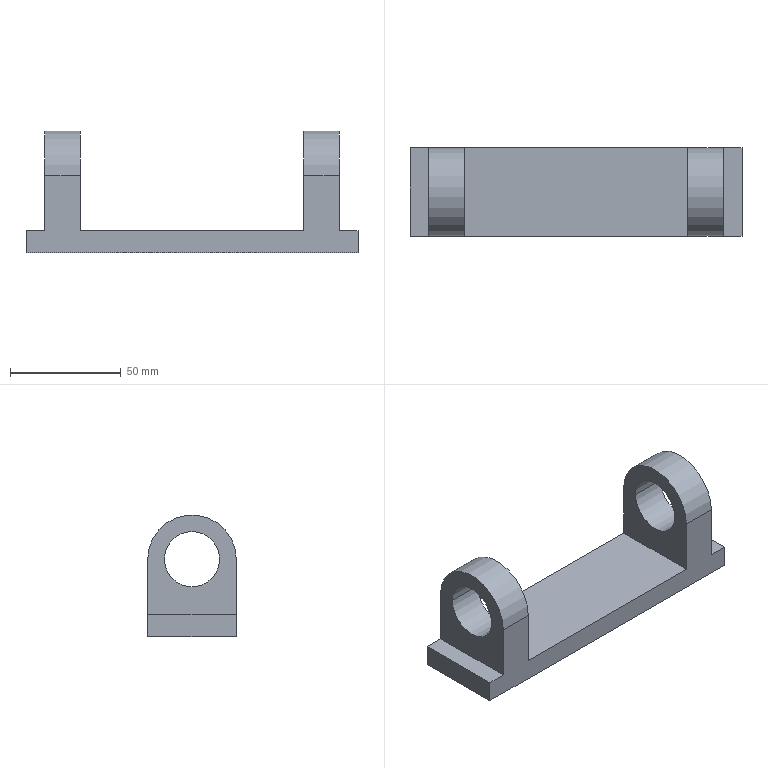Part | STEP file | TN-NHGJQJ-001-001 | 1 solid | 18 faces | box 150 x 40 x 55 mm | volume 96398 mm3 | plane 12 | cylinder 6 | commonest cylinder face diameters 25 x4 40 x2
STEP:
#1=CARTESIAN_POINT('',(61.678,18.702,35.));
#2=VERTEX_POINT('',#1);
#3=CARTESIAN_POINT('',(61.678,-6.298,35.));
#4=VERTEX_POINT('',#3);
#5=CARTESIAN_POINT('',(61.678,6.202,35.));
#6=DIRECTION('',(-1.,0.,0.));
#7=DIRECTION('',(0.,1.,0.));
#8=AXIS2_PLACEMENT_3D('',#5,#6,#7);
#9=CIRCLE('',#8,12.5);
#10=EDGE_CURVE('',#2,#4,#9,.T.);
#11=ORIENTED_EDGE('',*,*,#10,.T.);
#12=CARTESIAN_POINT('',(77.678,-6.298,35.));
#13=VERTEX_POINT('',#12);
#14=CARTESIAN_POINT('',(-63.822,-6.298,35.));
#15=DIRECTION('',(1.,0.,0.));
#16=VECTOR('',#15,1000.);
#17=LINE('',#14,#16);
#18=EDGE_CURVE('',#4,#13,#17,.T.);
#19=ORIENTED_EDGE('',*,*,#18,.T.);
#20=CARTESIAN_POINT('',(77.678,18.702,35.));
#21=VERTEX_POINT('',#20);
#22=CARTESIAN_POINT('',(77.678,6.202,35.));
#23=DIRECTION('',(1.,0.,0.));
#24=DIRECTION('',(0.,1.,0.));
#25=AXIS2_PLACEMENT_3D('',#22,#23,#24);
#26=CIRCLE('',#25,12.5);
#27=EDGE_CURVE('',#13,#21,#26,.T.);
#28=ORIENTED_EDGE('',*,*,#27,.T.);
#29=CARTESIAN_POINT('',(-63.822,18.702,35.));
#30=DIRECTION('',(1.,0.,0.));
#31=VECTOR('',#30,1000.);
#32=LINE('',#29,#31);
#33=EDGE_CURVE('',#2,#21,#32,.T.);
#34=ORIENTED_EDGE('',*,*,#33,.F.);
#35=EDGE_LOOP('',(#11,#19,#28,#34));
#36=FACE_OUTER_BOUND('',#35,.T.);
#37=CARTESIAN_POINT('',(-63.822,6.202,35.));
#38=DIRECTION('',(1.,0.,0.));
#39=DIRECTION('',(0.,1.,0.));
#40=AXIS2_PLACEMENT_3D('',#37,#38,#39);
#41=CYLINDRICAL_SURFACE('',#40,12.5);
#42=ADVANCED_FACE('',(#36),#41,.F.);
#43=CARTESIAN_POINT('',(-55.322,18.702,35.));
#44=VERTEX_POINT('',#43);
#45=CARTESIAN_POINT('',(-55.322,-6.298,35.));
#46=VERTEX_POINT('',#45);
#47=CARTESIAN_POINT('',(-55.322,6.202,35.));
#48=DIRECTION('',(-1.,0.,0.));
#49=DIRECTION('',(0.,1.,0.));
#50=AXIS2_PLACEMENT_3D('',#47,#48,#49);
#51=CIRCLE('',#50,12.5);
#52=EDGE_CURVE('',#44,#46,#51,.T.);
#53=ORIENTED_EDGE('',*,*,#52,.T.);
#54=CARTESIAN_POINT('',(-39.322,-6.298,35.));
#55=VERTEX_POINT('',#54);
#56=CARTESIAN_POINT('',(-63.822,-6.298,35.));
#57=DIRECTION('',(1.,0.,0.));
#58=VECTOR('',#57,1000.);
#59=LINE('',#56,#58);
#60=EDGE_CURVE('',#46,#55,#59,.T.);
#61=ORIENTED_EDGE('',*,*,#60,.T.);
#62=CARTESIAN_POINT('',(-39.322,18.702,35.));
#63=VERTEX_POINT('',#62);
#64=CARTESIAN_POINT('',(-39.322,6.202,35.));
#65=DIRECTION('',(1.,0.,0.));
#66=DIRECTION('',(0.,1.,0.));
#67=AXIS2_PLACEMENT_3D('',#64,#65,#66);
#68=CIRCLE('',#67,12.5);
#69=EDGE_CURVE('',#55,#63,#68,.T.);
#70=ORIENTED_EDGE('',*,*,#69,.T.);
#71=CARTESIAN_POINT('',(-63.822,18.702,35.));
#72=DIRECTION('',(1.,0.,0.));
#73=VECTOR('',#72,1000.);
#74=LINE('',#71,#73);
#75=EDGE_CURVE('',#44,#63,#74,.T.);
#76=ORIENTED_EDGE('',*,*,#75,.F.);
#77=EDGE_LOOP('',(#53,#61,#70,#76));
#78=FACE_OUTER_BOUND('',#77,.T.);
#79=CARTESIAN_POINT('',(-63.822,6.202,35.));
#80=DIRECTION('',(1.,0.,0.));
#81=DIRECTION('',(0.,1.,0.));
#82=AXIS2_PLACEMENT_3D('',#79,#80,#81);
#83=CYLINDRICAL_SURFACE('',#82,12.5);
#84=ADVANCED_FACE('',(#78),#83,.F.);
#85=CARTESIAN_POINT('',(86.178,26.202,0.));
#86=VERTEX_POINT('',#85);
#87=CARTESIAN_POINT('',(-63.822,26.202,0.));
#88=VERTEX_POINT('',#87);
#89=CARTESIAN_POINT('',(0.,26.202,0.));
#90=DIRECTION('',(-1.,0.,0.));
#91=VECTOR('',#90,1000.);
#92=LINE('',#89,#91);
#93=EDGE_CURVE('',#86,#88,#92,.T.);
#94=ORIENTED_EDGE('',*,*,#93,.F.);
#95=CARTESIAN_POINT('',(86.178,-13.798,0.));
#96=VERTEX_POINT('',#95);
#97=CARTESIAN_POINT('',(86.178,0.,0.));
#98=DIRECTION('',(0.,1.,0.));
#99=VECTOR('',#98,1000.);
#100=LINE('',#97,#99);
#101=EDGE_CURVE('',#96,#86,#100,.T.);
#102=ORIENTED_EDGE('',*,*,#101,.F.);
#103=CARTESIAN_POINT('',(-63.822,-13.798,0.));
#104=VERTEX_POINT('',#103);
#105=CARTESIAN_POINT('',(0.,-13.798,0.));
#106=DIRECTION('',(1.,0.,0.));
#107=VECTOR('',#106,1000.);
#108=LINE('',#105,#107);
#109=EDGE_CURVE('',#104,#96,#108,.T.);
#110=ORIENTED_EDGE('',*,*,#109,.F.);
#111=CARTESIAN_POINT('',(-63.822,0.,0.));
#112=DIRECTION('',(0.,-1.,0.));
#113=VECTOR('',#112,1000.);
#114=LINE('',#111,#113);
#115=EDGE_CURVE('',#88,#104,#114,.T.);
#116=ORIENTED_EDGE('',*,*,#115,.F.);
#117=EDGE_LOOP('',(#94,#102,#110,#116));
#118=FACE_OUTER_BOUND('',#117,.T.);
#119=CARTESIAN_POINT('',(0.,0.,0.));
#120=DIRECTION('',(0.,0.,1.));
#121=DIRECTION('',(1.,0.,0.));
#122=AXIS2_PLACEMENT_3D('',#119,#120,#121);
#123=PLANE('',#122);
#124=ADVANCED_FACE('',(#118),#123,.F.);
#125=CARTESIAN_POINT('',(-63.822,-13.798,10.));
#126=VERTEX_POINT('',#125);
#127=CARTESIAN_POINT('',(-63.822,-13.798,10.));
#128=DIRECTION('',(0.,0.,-1.));
#129=VECTOR('',#128,1000.);
#130=LINE('',#127,#129);
#131=EDGE_CURVE('',#126,#104,#130,.T.);
#132=ORIENTED_EDGE('',*,*,#131,.F.);
#133=CARTESIAN_POINT('',(-63.822,26.202,10.));
#134=VERTEX_POINT('',#133);
#135=CARTESIAN_POINT('',(-63.822,26.202,10.));
#136=DIRECTION('',(0.,-1.,0.));
#137=VECTOR('',#136,1000.);
#138=LINE('',#135,#137);
#139=EDGE_CURVE('',#134,#126,#138,.T.);
#140=ORIENTED_EDGE('',*,*,#139,.F.);
#141=CARTESIAN_POINT('',(-63.822,26.202,10.));
#142=DIRECTION('',(0.,0.,1.));
#143=VECTOR('',#142,1000.);
#144=LINE('',#141,#143);
#145=EDGE_CURVE('',#88,#134,#144,.T.);
#146=ORIENTED_EDGE('',*,*,#145,.F.);
#147=ORIENTED_EDGE('',*,*,#115,.T.);
#148=EDGE_LOOP('',(#132,#140,#146,#147));
#149=FACE_OUTER_BOUND('',#148,.T.);
#150=CARTESIAN_POINT('',(-63.822,26.202,10.));
#151=DIRECTION('',(1.,0.,0.));
#152=DIRECTION('',(0.,1.,0.));
#153=AXIS2_PLACEMENT_3D('',#150,#151,#152);
#154=PLANE('',#153);
#155=ADVANCED_FACE('',(#149),#154,.F.);
#156=CARTESIAN_POINT('',(77.678,26.202,35.));
#157=VERTEX_POINT('',#156);
#158=CARTESIAN_POINT('',(61.678,26.202,35.));
#159=VERTEX_POINT('',#158);
#160=CARTESIAN_POINT('',(-63.822,26.202,35.));
#161=DIRECTION('',(-1.,0.,0.));
#162=VECTOR('',#161,1000.);
#163=LINE('',#160,#162);
#164=EDGE_CURVE('',#157,#159,#163,.T.);
#165=ORIENTED_EDGE('',*,*,#164,.F.);
#166=CARTESIAN_POINT('',(77.678,26.202,10.));
#167=VERTEX_POINT('',#166);
#168=CARTESIAN_POINT('',(77.678,26.202,10.));
#169=DIRECTION('',(0.,0.,1.));
#170=VECTOR('',#169,1000.);
#171=LINE('',#168,#170);
#172=EDGE_CURVE('',#167,#157,#171,.T.);
#173=ORIENTED_EDGE('',*,*,#172,.F.);
#174=CARTESIAN_POINT('',(86.178,26.202,10.));
#175=VERTEX_POINT('',#174);
#176=CARTESIAN_POINT('',(-63.822,26.202,10.));
#177=DIRECTION('',(-1.,0.,0.));
#178=VECTOR('',#177,1000.);
#179=LINE('',#176,#178);
#180=EDGE_CURVE('',#175,#167,#179,.T.);
#181=ORIENTED_EDGE('',*,*,#180,.F.);
#182=CARTESIAN_POINT('',(86.178,26.202,10.));
#183=DIRECTION('',(0.,0.,1.));
#184=VECTOR('',#183,1000.);
#185=LINE('',#182,#184);
#186=EDGE_CURVE('',#86,#175,#185,.T.);
#187=ORIENTED_EDGE('',*,*,#186,.F.);
#188=ORIENTED_EDGE('',*,*,#93,.T.);
#189=ORIENTED_EDGE('',*,*,#145,.T.);
#190=CARTESIAN_POINT('',(-55.322,26.202,10.));
#191=VERTEX_POINT('',#190);
#192=CARTESIAN_POINT('',(-63.822,26.202,10.));
#193=DIRECTION('',(-1.,0.,0.));
#194=VECTOR('',#193,1000.);
#195=LINE('',#192,#194);
#196=EDGE_CURVE('',#191,#134,#195,.T.);
#197=ORIENTED_EDGE('',*,*,#196,.F.);
#198=CARTESIAN_POINT('',(-55.322,26.202,35.));
#199=VERTEX_POINT('',#198);
#200=CARTESIAN_POINT('',(-55.322,26.202,10.));
#201=DIRECTION('',(0.,0.,-1.));
#202=VECTOR('',#201,1000.);
#203=LINE('',#200,#202);
#204=EDGE_CURVE('',#199,#191,#203,.T.);
#205=ORIENTED_EDGE('',*,*,#204,.F.);
#206=CARTESIAN_POINT('',(-39.322,26.202,35.));
#207=VERTEX_POINT('',#206);
#208=CARTESIAN_POINT('',(-63.822,26.202,35.));
#209=DIRECTION('',(-1.,0.,0.));
#210=VECTOR('',#209,1000.);
#211=LINE('',#208,#210);
#212=EDGE_CURVE('',#207,#199,#211,.T.);
#213=ORIENTED_EDGE('',*,*,#212,.F.);
#214=CARTESIAN_POINT('',(-39.322,26.202,10.));
#215=VERTEX_POINT('',#214);
#216=CARTESIAN_POINT('',(-39.322,26.202,10.));
#217=DIRECTION('',(0.,0.,1.));
#218=VECTOR('',#217,1000.);
#219=LINE('',#216,#218);
#220=EDGE_CURVE('',#215,#207,#219,.T.);
#221=ORIENTED_EDGE('',*,*,#220,.F.);
#222=CARTESIAN_POINT('',(61.678,26.202,10.));
#223=VERTEX_POINT('',#222);
#224=CARTESIAN_POINT('',(-63.822,26.202,10.));
#225=DIRECTION('',(-1.,0.,0.));
#226=VECTOR('',#225,1000.);
#227=LINE('',#224,#226);
#228=EDGE_CURVE('',#223,#215,#227,.T.);
#229=ORIENTED_EDGE('',*,*,#228,.F.);
#230=CARTESIAN_POINT('',(61.678,26.202,10.));
#231=DIRECTION('',(0.,0.,-1.));
#232=VECTOR('',#231,1000.);
#233=LINE('',#230,#232);
#234=EDGE_CURVE('',#159,#223,#233,.T.);
#235=ORIENTED_EDGE('',*,*,#234,.F.);
#236=EDGE_LOOP('',(#165,#173,#181,#187,#188,#189,#197,#205,#213,#221,#229,#235));
#237=FACE_OUTER_BOUND('',#236,.T.);
#238=CARTESIAN_POINT('',(-63.822,26.202,10.));
#239=DIRECTION('',(0.,-1.,0.));
#240=DIRECTION('',(0.,0.,-1.));
#241=AXIS2_PLACEMENT_3D('',#238,#239,#240);
#242=PLANE('',#241);
#243=ADVANCED_FACE('',(#237),#242,.F.);
#244=ORIENTED_EDGE('',*,*,#186,.T.);
#245=CARTESIAN_POINT('',(86.178,-13.798,10.));
#246=VERTEX_POINT('',#245);
#247=CARTESIAN_POINT('',(86.178,26.202,10.));
#248=DIRECTION('',(0.,1.,0.));
#249=VECTOR('',#248,1000.);
#250=LINE('',#247,#249);
#251=EDGE_CURVE('',#246,#175,#250,.T.);
#252=ORIENTED_EDGE('',*,*,#251,.F.);
#253=CARTESIAN_POINT('',(86.178,-13.798,10.));
#254=DIRECTION('',(0.,0.,1.));
#255=VECTOR('',#254,1000.);
#256=LINE('',#253,#255);
#257=EDGE_CURVE('',#96,#246,#256,.T.);
#258=ORIENTED_EDGE('',*,*,#257,.F.);
#259=ORIENTED_EDGE('',*,*,#101,.T.);
#260=EDGE_LOOP('',(#244,#252,#258,#259));
#261=FACE_OUTER_BOUND('',#260,.T.);
#262=CARTESIAN_POINT('',(86.178,26.202,10.));
#263=DIRECTION('',(-1.,0.,0.));
#264=DIRECTION('',(0.,0.,1.));
#265=AXIS2_PLACEMENT_3D('',#262,#263,#264);
#266=PLANE('',#265);
#267=ADVANCED_FACE('',(#261),#266,.F.);
#268=CARTESIAN_POINT('',(61.678,-13.798,35.));
#269=VERTEX_POINT('',#268);
#270=CARTESIAN_POINT('',(77.678,-13.798,35.));
#271=VERTEX_POINT('',#270);
#272=CARTESIAN_POINT('',(-63.822,-13.798,35.));
#273=DIRECTION('',(1.,0.,0.));
#274=VECTOR('',#273,1000.);
#275=LINE('',#272,#274);
#276=EDGE_CURVE('',#269,#271,#275,.T.);
#277=ORIENTED_EDGE('',*,*,#276,.F.);
#278=CARTESIAN_POINT('',(61.678,-13.798,10.));
#279=VERTEX_POINT('',#278);
#280=CARTESIAN_POINT('',(61.678,-13.798,10.));
#281=DIRECTION('',(0.,0.,1.));
#282=VECTOR('',#281,1000.);
#283=LINE('',#280,#282);
#284=EDGE_CURVE('',#279,#269,#283,.T.);
#285=ORIENTED_EDGE('',*,*,#284,.F.);
#286=CARTESIAN_POINT('',(-39.322,-13.798,10.));
#287=VERTEX_POINT('',#286);
#288=CARTESIAN_POINT('',(-63.822,-13.798,10.));
#289=DIRECTION('',(1.,0.,0.));
#290=VECTOR('',#289,1000.);
#291=LINE('',#288,#290);
#292=EDGE_CURVE('',#287,#279,#291,.T.);
#293=ORIENTED_EDGE('',*,*,#292,.F.);
#294=CARTESIAN_POINT('',(-39.322,-13.798,35.));
#295=VERTEX_POINT('',#294);
#296=CARTESIAN_POINT('',(-39.322,-13.798,10.));
#297=DIRECTION('',(0.,0.,-1.));
#298=VECTOR('',#297,1000.);
#299=LINE('',#296,#298);
#300=EDGE_CURVE('',#295,#287,#299,.T.);
#301=ORIENTED_EDGE('',*,*,#300,.F.);
#302=CARTESIAN_POINT('',(-55.322,-13.798,35.));
#303=VERTEX_POINT('',#302);
#304=CARTESIAN_POINT('',(-63.822,-13.798,35.));
#305=DIRECTION('',(1.,0.,0.));
#306=VECTOR('',#305,1000.);
#307=LINE('',#304,#306);
#308=EDGE_CURVE('',#303,#295,#307,.T.);
#309=ORIENTED_EDGE('',*,*,#308,.F.);
#310=CARTESIAN_POINT('',(-55.322,-13.798,10.));
#311=VERTEX_POINT('',#310);
#312=CARTESIAN_POINT('',(-55.322,-13.798,10.));
#313=DIRECTION('',(0.,0.,1.));
#314=VECTOR('',#313,1000.);
#315=LINE('',#312,#314);
#316=EDGE_CURVE('',#311,#303,#315,.T.);
#317=ORIENTED_EDGE('',*,*,#316,.F.);
#318=CARTESIAN_POINT('',(-63.822,-13.798,10.));
#319=DIRECTION('',(1.,0.,0.));
#320=VECTOR('',#319,1000.);
#321=LINE('',#318,#320);
#322=EDGE_CURVE('',#126,#311,#321,.T.);
#323=ORIENTED_EDGE('',*,*,#322,.F.);
#324=ORIENTED_EDGE('',*,*,#131,.T.);
#325=ORIENTED_EDGE('',*,*,#109,.T.);
#326=ORIENTED_EDGE('',*,*,#257,.T.);
#327=CARTESIAN_POINT('',(77.678,-13.798,10.));
#328=VERTEX_POINT('',#327);
#329=CARTESIAN_POINT('',(-63.822,-13.798,10.));
#330=DIRECTION('',(1.,0.,0.));
#331=VECTOR('',#330,1000.);
#332=LINE('',#329,#331);
#333=EDGE_CURVE('',#328,#246,#332,.T.);
#334=ORIENTED_EDGE('',*,*,#333,.F.);
#335=CARTESIAN_POINT('',(77.678,-13.798,10.));
#336=DIRECTION('',(0.,0.,-1.));
#337=VECTOR('',#336,1000.);
#338=LINE('',#335,#337);
#339=EDGE_CURVE('',#271,#328,#338,.T.);
#340=ORIENTED_EDGE('',*,*,#339,.F.);
#341=EDGE_LOOP('',(#277,#285,#293,#301,#309,#317,#323,#324,#325,#326,#334,#340));
#342=FACE_OUTER_BOUND('',#341,.T.);
#343=CARTESIAN_POINT('',(-63.822,-13.798,10.));
#344=DIRECTION('',(0.,1.,0.));
#345=DIRECTION('',(0.,0.,1.));
#346=AXIS2_PLACEMENT_3D('',#343,#344,#345);
#347=PLANE('',#346);
#348=ADVANCED_FACE('',(#342),#347,.F.);
#349=ORIENTED_EDGE('',*,*,#139,.T.);
#350=ORIENTED_EDGE('',*,*,#322,.T.);
#351=CARTESIAN_POINT('',(-55.322,0.,10.));
#352=DIRECTION('',(0.,1.,0.));
#353=VECTOR('',#352,1000.);
#354=LINE('',#351,#353);
#355=EDGE_CURVE('',#311,#191,#354,.T.);
#356=ORIENTED_EDGE('',*,*,#355,.T.);
#357=ORIENTED_EDGE('',*,*,#196,.T.);
#358=EDGE_LOOP('',(#349,#350,#356,#357));
#359=FACE_OUTER_BOUND('',#358,.T.);
#360=CARTESIAN_POINT('',(0.,0.,10.));
#361=DIRECTION('',(0.,0.,1.));
#362=DIRECTION('',(1.,0.,0.));
#363=AXIS2_PLACEMENT_3D('',#360,#361,#362);
#364=PLANE('',#363);
#365=ADVANCED_FACE('',(#359),#364,.T.);
#366=CARTESIAN_POINT('',(61.678,6.202,35.));
#367=DIRECTION('',(1.,0.,0.));
#368=DIRECTION('',(0.,0.,1.));
#369=AXIS2_PLACEMENT_3D('',#366,#367,#368);
#370=CIRCLE('',#369,20.);
#371=EDGE_CURVE('',#159,#269,#370,.T.);
#372=ORIENTED_EDGE('',*,*,#371,.F.);
#373=ORIENTED_EDGE('',*,*,#234,.T.);
#374=CARTESIAN_POINT('',(61.678,26.202,10.));
#375=DIRECTION('',(0.,1.,0.));
#376=VECTOR('',#375,1000.);
#377=LINE('',#374,#376);
#378=EDGE_CURVE('',#279,#223,#377,.T.);
#379=ORIENTED_EDGE('',*,*,#378,.F.);
#380=ORIENTED_EDGE('',*,*,#284,.T.);
#381=EDGE_LOOP('',(#372,#373,#379,#380));
#382=FACE_OUTER_BOUND('',#381,.T.);
#383=ORIENTED_EDGE('',*,*,#10,.F.);
#384=CARTESIAN_POINT('',(61.678,6.202,35.));
#385=DIRECTION('',(-1.,0.,0.));
#386=DIRECTION('',(0.,1.,0.));
#387=AXIS2_PLACEMENT_3D('',#384,#385,#386);
#388=CIRCLE('',#387,12.5);
#389=EDGE_CURVE('',#4,#2,#388,.T.);
#390=ORIENTED_EDGE('',*,*,#389,.F.);
#391=EDGE_LOOP('',(#383,#390));
#392=FACE_BOUND('',#391,.T.);
#393=CARTESIAN_POINT('',(61.678,26.202,55.));
#394=DIRECTION('',(1.,0.,0.));
#395=DIRECTION('',(0.,1.,0.));
#396=AXIS2_PLACEMENT_3D('',#393,#394,#395);
#397=PLANE('',#396);
#398=ADVANCED_FACE('',(#382,#392),#397,.F.);
#399=ORIENTED_EDGE('',*,*,#164,.T.);
#400=ORIENTED_EDGE('',*,*,#371,.T.);
#401=ORIENTED_EDGE('',*,*,#276,.T.);
#402=CARTESIAN_POINT('',(77.678,6.202,35.));
#403=DIRECTION('',(-1.,0.,0.));
#404=DIRECTION('',(0.,0.,-1.));
#405=AXIS2_PLACEMENT_3D('',#402,#403,#404);
#406=CIRCLE('',#405,20.);
#407=EDGE_CURVE('',#271,#157,#406,.T.);
#408=ORIENTED_EDGE('',*,*,#407,.T.);
#409=EDGE_LOOP('',(#399,#400,#401,#408));
#410=FACE_OUTER_BOUND('',#409,.T.);
#411=CARTESIAN_POINT('',(0.,6.202,35.));
#412=DIRECTION('',(1.,0.,0.));
#413=DIRECTION('',(0.,0.,-1.));
#414=AXIS2_PLACEMENT_3D('',#411,#412,#413);
#415=CYLINDRICAL_SURFACE('',#414,20.);
#416=ADVANCED_FACE('',(#410),#415,.T.);
#417=ORIENTED_EDGE('',*,*,#407,.F.);
#418=ORIENTED_EDGE('',*,*,#339,.T.);
#419=CARTESIAN_POINT('',(77.678,26.202,10.));
#420=DIRECTION('',(0.,-1.,0.));
#421=VECTOR('',#420,1000.);
#422=LINE('',#419,#421);
#423=EDGE_CURVE('',#167,#328,#422,.T.);
#424=ORIENTED_EDGE('',*,*,#423,.F.);
#425=ORIENTED_EDGE('',*,*,#172,.T.);
#426=EDGE_LOOP('',(#417,#418,#424,#425));
#427=FACE_OUTER_BOUND('',#426,.T.);
#428=CARTESIAN_POINT('',(77.678,6.202,35.));
#429=DIRECTION('',(1.,0.,0.));
#430=DIRECTION('',(0.,1.,0.));
#431=AXIS2_PLACEMENT_3D('',#428,#429,#430);
#432=CIRCLE('',#431,12.5);
#433=EDGE_CURVE('',#21,#13,#432,.T.);
#434=ORIENTED_EDGE('',*,*,#433,.F.);
#435=ORIENTED_EDGE('',*,*,#27,.F.);
#436=EDGE_LOOP('',(#434,#435));
#437=FACE_BOUND('',#436,.T.);
#438=CARTESIAN_POINT('',(77.678,26.202,55.));
#439=DIRECTION('',(-1.,0.,0.));
#440=DIRECTION('',(0.,-1.,0.));
#441=AXIS2_PLACEMENT_3D('',#438,#439,#440);
#442=PLANE('',#441);
#443=ADVANCED_FACE('',(#427,#437),#442,.F.);
#444=ORIENTED_EDGE('',*,*,#333,.T.);
#445=ORIENTED_EDGE('',*,*,#251,.T.);
#446=ORIENTED_EDGE('',*,*,#180,.T.);
#447=ORIENTED_EDGE('',*,*,#423,.T.);
#448=EDGE_LOOP('',(#444,#445,#446,#447));
#449=FACE_OUTER_BOUND('',#448,.T.);
#450=CARTESIAN_POINT('',(0.,0.,10.));
#451=DIRECTION('',(0.,0.,1.));
#452=DIRECTION('',(1.,0.,0.));
#453=AXIS2_PLACEMENT_3D('',#450,#451,#452);
#454=PLANE('',#453);
#455=ADVANCED_FACE('',(#449),#454,.T.);
#456=CARTESIAN_POINT('',(-55.322,6.202,35.));
#457=DIRECTION('',(1.,0.,0.));
#458=DIRECTION('',(0.,0.,1.));
#459=AXIS2_PLACEMENT_3D('',#456,#457,#458);
#460=CIRCLE('',#459,20.);
#461=EDGE_CURVE('',#199,#303,#460,.T.);
#462=ORIENTED_EDGE('',*,*,#461,.F.);
#463=ORIENTED_EDGE('',*,*,#204,.T.);
#464=ORIENTED_EDGE('',*,*,#355,.F.);
#465=ORIENTED_EDGE('',*,*,#316,.T.);
#466=EDGE_LOOP('',(#462,#463,#464,#465));
#467=FACE_OUTER_BOUND('',#466,.T.);
#468=ORIENTED_EDGE('',*,*,#52,.F.);
#469=CARTESIAN_POINT('',(-55.322,6.202,35.));
#470=DIRECTION('',(-1.,0.,0.));
#471=DIRECTION('',(0.,1.,0.));
#472=AXIS2_PLACEMENT_3D('',#469,#470,#471);
#473=CIRCLE('',#472,12.5);
#474=EDGE_CURVE('',#46,#44,#473,.T.);
#475=ORIENTED_EDGE('',*,*,#474,.F.);
#476=EDGE_LOOP('',(#468,#475));
#477=FACE_BOUND('',#476,.T.);
#478=CARTESIAN_POINT('',(-55.322,26.202,55.));
#479=DIRECTION('',(1.,0.,0.));
#480=DIRECTION('',(0.,0.,-1.));
#481=AXIS2_PLACEMENT_3D('',#478,#479,#480);
#482=PLANE('',#481);
#483=ADVANCED_FACE('',(#467,#477),#482,.F.);
#484=ORIENTED_EDGE('',*,*,#212,.T.);
#485=ORIENTED_EDGE('',*,*,#461,.T.);
#486=ORIENTED_EDGE('',*,*,#308,.T.);
#487=CARTESIAN_POINT('',(-39.322,6.202,35.));
#488=DIRECTION('',(-1.,0.,0.));
#489=DIRECTION('',(0.,0.,-1.));
#490=AXIS2_PLACEMENT_3D('',#487,#488,#489);
#491=CIRCLE('',#490,20.);
#492=EDGE_CURVE('',#295,#207,#491,.T.);
#493=ORIENTED_EDGE('',*,*,#492,.T.);
#494=EDGE_LOOP('',(#484,#485,#486,#493));
#495=FACE_OUTER_BOUND('',#494,.T.);
#496=CARTESIAN_POINT('',(0.,6.202,35.));
#497=DIRECTION('',(1.,0.,0.));
#498=DIRECTION('',(0.,0.,-1.));
#499=AXIS2_PLACEMENT_3D('',#496,#497,#498);
#500=CYLINDRICAL_SURFACE('',#499,20.);
#501=ADVANCED_FACE('',(#495),#500,.T.);
#502=ORIENTED_EDGE('',*,*,#492,.F.);
#503=ORIENTED_EDGE('',*,*,#300,.T.);
#504=CARTESIAN_POINT('',(-39.322,26.202,10.));
#505=DIRECTION('',(0.,-1.,0.));
#506=VECTOR('',#505,1000.);
#507=LINE('',#504,#506);
#508=EDGE_CURVE('',#215,#287,#507,.T.);
#509=ORIENTED_EDGE('',*,*,#508,.F.);
#510=ORIENTED_EDGE('',*,*,#220,.T.);
#511=EDGE_LOOP('',(#502,#503,#509,#510));
#512=FACE_OUTER_BOUND('',#511,.T.);
#513=CARTESIAN_POINT('',(-39.322,6.202,35.));
#514=DIRECTION('',(1.,0.,0.));
#515=DIRECTION('',(0.,1.,0.));
#516=AXIS2_PLACEMENT_3D('',#513,#514,#515);
#517=CIRCLE('',#516,12.5);
#518=EDGE_CURVE('',#63,#55,#517,.T.);
#519=ORIENTED_EDGE('',*,*,#518,.F.);
#520=ORIENTED_EDGE('',*,*,#69,.F.);
#521=EDGE_LOOP('',(#519,#520));
#522=FACE_BOUND('',#521,.T.);
#523=CARTESIAN_POINT('',(-39.322,26.202,55.));
#524=DIRECTION('',(-1.,0.,0.));
#525=DIRECTION('',(0.,-1.,0.));
#526=AXIS2_PLACEMENT_3D('',#523,#524,#525);
#527=PLANE('',#526);
#528=ADVANCED_FACE('',(#512,#522),#527,.F.);
#529=ORIENTED_EDGE('',*,*,#228,.T.);
#530=ORIENTED_EDGE('',*,*,#508,.T.);
#531=ORIENTED_EDGE('',*,*,#292,.T.);
#532=ORIENTED_EDGE('',*,*,#378,.T.);
#533=EDGE_LOOP('',(#529,#530,#531,#532));
#534=FACE_OUTER_BOUND('',#533,.T.);
#535=CARTESIAN_POINT('',(0.,0.,10.));
#536=DIRECTION('',(0.,0.,1.));
#537=DIRECTION('',(1.,0.,0.));
#538=AXIS2_PLACEMENT_3D('',#535,#536,#537);
#539=PLANE('',#538);
#540=ADVANCED_FACE('',(#534),#539,.T.);
#541=ORIENTED_EDGE('',*,*,#18,.F.);
#542=ORIENTED_EDGE('',*,*,#389,.T.);
#543=ORIENTED_EDGE('',*,*,#33,.T.);
#544=ORIENTED_EDGE('',*,*,#433,.T.);
#545=EDGE_LOOP('',(#541,#542,#543,#544));
#546=FACE_OUTER_BOUND('',#545,.T.);
#547=CARTESIAN_POINT('',(-63.822,6.202,35.));
#548=DIRECTION('',(1.,0.,0.));
#549=DIRECTION('',(0.,1.,0.));
#550=AXIS2_PLACEMENT_3D('',#547,#548,#549);
#551=CYLINDRICAL_SURFACE('',#550,12.5);
#552=ADVANCED_FACE('',(#546),#551,.F.);
#553=ORIENTED_EDGE('',*,*,#60,.F.);
#554=ORIENTED_EDGE('',*,*,#474,.T.);
#555=ORIENTED_EDGE('',*,*,#75,.T.);
#556=ORIENTED_EDGE('',*,*,#518,.T.);
#557=EDGE_LOOP('',(#553,#554,#555,#556));
#558=FACE_OUTER_BOUND('',#557,.T.);
#559=CARTESIAN_POINT('',(-63.822,6.202,35.));
#560=DIRECTION('',(1.,0.,0.));
#561=DIRECTION('',(0.,1.,0.));
#562=AXIS2_PLACEMENT_3D('',#559,#560,#561);
#563=CYLINDRICAL_SURFACE('',#562,12.5);
#564=ADVANCED_FACE('',(#558),#563,.F.);
#565=CLOSED_SHELL('',(#42,#84,#124,#155,#243,#267,#348,#365,#398,#416,#443,#455,#483,#501,#528,#540,#552,#564));
#566=MANIFOLD_SOLID_BREP('',#565);
#567=CARTESIAN_POINT('',(0.,0.,0.));
#568=DIRECTION('',(0.,0.,1.));
#569=DIRECTION('',(1.,0.,0.));
#570=AXIS2_PLACEMENT_3D('',#567,#568,#569);
#571=(LENGTH_UNIT()NAMED_UNIT(*)SI_UNIT(.MILLI.,.METRE.));
#572=UNCERTAINTY_MEASURE_WITH_UNIT(LENGTH_MEASURE(0.00001),#571,'','');
#573=(NAMED_UNIT(*)PLANE_ANGLE_UNIT()SI_UNIT($,.RADIAN.));
#574=(NAMED_UNIT(*)SI_UNIT($,.STERADIAN.)SOLID_ANGLE_UNIT());
#575=(GEOMETRIC_REPRESENTATION_CONTEXT(3)GLOBAL_UNCERTAINTY_ASSIGNED_CONTEXT((#572))GLOBAL_UNIT_ASSIGNED_CONTEXT((#571,#573,#574))REPRESENTATION_CONTEXT('',''));
#576=ADVANCED_BREP_SHAPE_REPRESENTATION('',(#566,#570),#575);